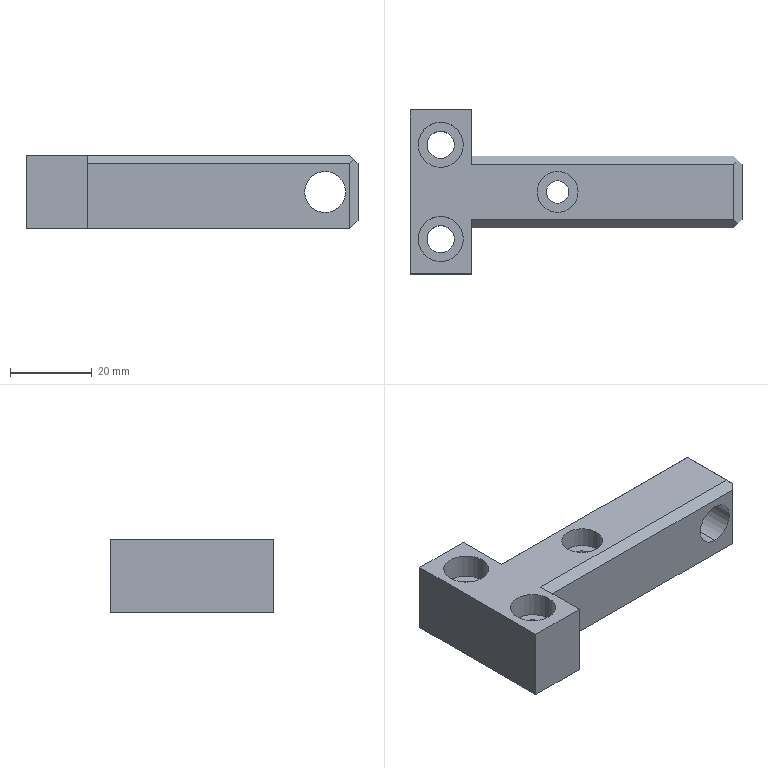Part | NX | features BREP 1 | 1 solid | 33 faces | box 81 x 40 x 18 mm | volume 27164 mm3 | plane 19 | cylinder 14 | commonest cylinder face diameters 6.6 x4 10 x4 11 x4 5.5 x2
STEP:
#1=CARTESIAN_POINT('',(17.428,-446.677,13.));
#2=VERTEX_POINT('',#1);
#3=CARTESIAN_POINT('',(27.428,-446.677,13.));
#4=VERTEX_POINT('',#3);
#5=CARTESIAN_POINT('',(22.428,-446.677,13.));
#6=DIRECTION('',(0.,0.,1.));
#7=DIRECTION('',(1.,0.,0.));
#8=AXIS2_PLACEMENT_3D('',#5,#6,#7);
#9=CIRCLE('',#8,5.);
#10=EDGE_CURVE('',#2,#4,#9,.T.);
#11=ORIENTED_EDGE('',*,*,#10,.F.);
#12=CARTESIAN_POINT('',(17.428,-446.677,18.));
#13=VERTEX_POINT('',#12);
#14=CARTESIAN_POINT('',(17.428,-446.677,18.));
#15=DIRECTION('',(0.,0.,1.));
#16=VECTOR('',#15,1000.);
#17=LINE('',#14,#16);
#18=EDGE_CURVE('',#13,#2,#17,.F.);
#19=ORIENTED_EDGE('',*,*,#18,.F.);
#20=CARTESIAN_POINT('',(27.428,-446.677,18.));
#21=VERTEX_POINT('',#20);
#22=CARTESIAN_POINT('',(22.428,-446.677,18.));
#23=DIRECTION('',(0.,0.,1.));
#24=DIRECTION('',(1.,0.,0.));
#25=AXIS2_PLACEMENT_3D('',#22,#23,#24);
#26=CIRCLE('',#25,5.);
#27=EDGE_CURVE('',#13,#21,#26,.T.);
#28=ORIENTED_EDGE('',*,*,#27,.T.);
#29=CARTESIAN_POINT('',(27.428,-446.677,18.));
#30=DIRECTION('',(0.,0.,1.));
#31=VECTOR('',#30,1000.);
#32=LINE('',#29,#31);
#33=EDGE_CURVE('',#21,#4,#32,.F.);
#34=ORIENTED_EDGE('',*,*,#33,.T.);
#35=EDGE_LOOP('',(#11,#19,#28,#34));
#36=FACE_BOUND('',#35,.T.);
#37=CARTESIAN_POINT('',(22.428,-446.677,18.));
#38=DIRECTION('',(0.,0.,1.));
#39=DIRECTION('',(1.,0.,0.));
#40=AXIS2_PLACEMENT_3D('',#37,#38,#39);
#41=CYLINDRICAL_SURFACE('',#40,5.);
#42=ADVANCED_FACE('',(#36),#41,.F.);
#43=CARTESIAN_POINT('',(19.678,-446.677,0.));
#44=VERTEX_POINT('',#43);
#45=CARTESIAN_POINT('',(25.178,-446.677,0.));
#46=VERTEX_POINT('',#45);
#47=CARTESIAN_POINT('',(22.428,-446.677,0.));
#48=DIRECTION('',(0.,0.,1.));
#49=DIRECTION('',(1.,0.,0.));
#50=AXIS2_PLACEMENT_3D('',#47,#48,#49);
#51=CIRCLE('',#50,2.75);
#52=EDGE_CURVE('',#44,#46,#51,.T.);
#53=ORIENTED_EDGE('',*,*,#52,.F.);
#54=CARTESIAN_POINT('',(19.678,-446.677,13.));
#55=VERTEX_POINT('',#54);
#56=CARTESIAN_POINT('',(19.678,-446.677,18.));
#57=DIRECTION('',(0.,0.,1.));
#58=VECTOR('',#57,1000.);
#59=LINE('',#56,#58);
#60=EDGE_CURVE('',#55,#44,#59,.F.);
#61=ORIENTED_EDGE('',*,*,#60,.F.);
#62=CARTESIAN_POINT('',(25.178,-446.677,13.));
#63=VERTEX_POINT('',#62);
#64=CARTESIAN_POINT('',(22.428,-446.677,13.));
#65=DIRECTION('',(0.,0.,1.));
#66=DIRECTION('',(1.,0.,0.));
#67=AXIS2_PLACEMENT_3D('',#64,#65,#66);
#68=CIRCLE('',#67,2.75);
#69=EDGE_CURVE('',#55,#63,#68,.T.);
#70=ORIENTED_EDGE('',*,*,#69,.T.);
#71=CARTESIAN_POINT('',(25.178,-446.677,18.));
#72=DIRECTION('',(0.,0.,1.));
#73=VECTOR('',#72,1000.);
#74=LINE('',#71,#73);
#75=EDGE_CURVE('',#63,#46,#74,.F.);
#76=ORIENTED_EDGE('',*,*,#75,.T.);
#77=EDGE_LOOP('',(#53,#61,#70,#76));
#78=FACE_BOUND('',#77,.T.);
#79=CARTESIAN_POINT('',(22.428,-446.677,18.));
#80=DIRECTION('',(0.,0.,1.));
#81=DIRECTION('',(1.,0.,0.));
#82=AXIS2_PLACEMENT_3D('',#79,#80,#81);
#83=CYLINDRICAL_SURFACE('',#82,2.75);
#84=ADVANCED_FACE('',(#78),#83,.F.);
#85=CARTESIAN_POINT('',(-11.572,-435.177,12.));
#86=VERTEX_POINT('',#85);
#87=CARTESIAN_POINT('',(-0.5719,-435.177,12.));
#88=VERTEX_POINT('',#87);
#89=CARTESIAN_POINT('',(-6.072,-435.177,12.));
#90=DIRECTION('',(0.,0.,1.));
#91=DIRECTION('',(1.,0.,0.));
#92=AXIS2_PLACEMENT_3D('',#89,#90,#91);
#93=CIRCLE('',#92,5.5);
#94=EDGE_CURVE('',#86,#88,#93,.T.);
#95=ORIENTED_EDGE('',*,*,#94,.F.);
#96=CARTESIAN_POINT('',(-11.572,-435.177,18.));
#97=VERTEX_POINT('',#96);
#98=CARTESIAN_POINT('',(-11.572,-435.177,18.));
#99=DIRECTION('',(0.,0.,1.));
#100=VECTOR('',#99,1000.);
#101=LINE('',#98,#100);
#102=EDGE_CURVE('',#97,#86,#101,.F.);
#103=ORIENTED_EDGE('',*,*,#102,.F.);
#104=CARTESIAN_POINT('',(-0.5719,-435.177,18.));
#105=VERTEX_POINT('',#104);
#106=CARTESIAN_POINT('',(-6.072,-435.177,18.));
#107=DIRECTION('',(0.,0.,1.));
#108=DIRECTION('',(1.,0.,0.));
#109=AXIS2_PLACEMENT_3D('',#106,#107,#108);
#110=CIRCLE('',#109,5.5);
#111=EDGE_CURVE('',#97,#105,#110,.T.);
#112=ORIENTED_EDGE('',*,*,#111,.T.);
#113=CARTESIAN_POINT('',(-0.5719,-435.177,18.));
#114=DIRECTION('',(0.,0.,1.));
#115=VECTOR('',#114,1000.);
#116=LINE('',#113,#115);
#117=EDGE_CURVE('',#105,#88,#116,.F.);
#118=ORIENTED_EDGE('',*,*,#117,.T.);
#119=EDGE_LOOP('',(#95,#103,#112,#118));
#120=FACE_BOUND('',#119,.T.);
#121=CARTESIAN_POINT('',(-6.072,-435.177,18.));
#122=DIRECTION('',(0.,0.,1.));
#123=DIRECTION('',(1.,0.,0.));
#124=AXIS2_PLACEMENT_3D('',#121,#122,#123);
#125=CYLINDRICAL_SURFACE('',#124,5.5);
#126=ADVANCED_FACE('',(#120),#125,.F.);
#127=CARTESIAN_POINT('',(-9.372,-435.177,0.));
#128=VERTEX_POINT('',#127);
#129=CARTESIAN_POINT('',(-2.772,-435.177,0.));
#130=VERTEX_POINT('',#129);
#131=CARTESIAN_POINT('',(-6.072,-435.177,0.));
#132=DIRECTION('',(0.,0.,1.));
#133=DIRECTION('',(1.,0.,0.));
#134=AXIS2_PLACEMENT_3D('',#131,#132,#133);
#135=CIRCLE('',#134,3.3);
#136=EDGE_CURVE('',#128,#130,#135,.T.);
#137=ORIENTED_EDGE('',*,*,#136,.F.);
#138=CARTESIAN_POINT('',(-9.372,-435.177,12.));
#139=VERTEX_POINT('',#138);
#140=CARTESIAN_POINT('',(-9.372,-435.177,18.));
#141=DIRECTION('',(0.,0.,1.));
#142=VECTOR('',#141,1000.);
#143=LINE('',#140,#142);
#144=EDGE_CURVE('',#139,#128,#143,.F.);
#145=ORIENTED_EDGE('',*,*,#144,.F.);
#146=CARTESIAN_POINT('',(-2.772,-435.177,12.));
#147=VERTEX_POINT('',#146);
#148=CARTESIAN_POINT('',(-6.072,-435.177,12.));
#149=DIRECTION('',(0.,0.,1.));
#150=DIRECTION('',(1.,0.,0.));
#151=AXIS2_PLACEMENT_3D('',#148,#149,#150);
#152=CIRCLE('',#151,3.3);
#153=EDGE_CURVE('',#139,#147,#152,.T.);
#154=ORIENTED_EDGE('',*,*,#153,.T.);
#155=CARTESIAN_POINT('',(-2.772,-435.177,18.));
#156=DIRECTION('',(0.,0.,1.));
#157=VECTOR('',#156,1000.);
#158=LINE('',#155,#157);
#159=EDGE_CURVE('',#147,#130,#158,.F.);
#160=ORIENTED_EDGE('',*,*,#159,.T.);
#161=EDGE_LOOP('',(#137,#145,#154,#160));
#162=FACE_BOUND('',#161,.T.);
#163=CARTESIAN_POINT('',(-6.072,-435.177,18.));
#164=DIRECTION('',(0.,0.,1.));
#165=DIRECTION('',(1.,0.,0.));
#166=AXIS2_PLACEMENT_3D('',#163,#164,#165);
#167=CYLINDRICAL_SURFACE('',#166,3.3);
#168=ADVANCED_FACE('',(#162),#167,.F.);
#169=CARTESIAN_POINT('',(-11.572,-458.177,12.));
#170=VERTEX_POINT('',#169);
#171=CARTESIAN_POINT('',(-0.5719,-458.177,12.));
#172=VERTEX_POINT('',#171);
#173=CARTESIAN_POINT('',(-6.072,-458.177,12.));
#174=DIRECTION('',(0.,0.,1.));
#175=DIRECTION('',(1.,0.,0.));
#176=AXIS2_PLACEMENT_3D('',#173,#174,#175);
#177=CIRCLE('',#176,5.5);
#178=EDGE_CURVE('',#170,#172,#177,.T.);
#179=ORIENTED_EDGE('',*,*,#178,.F.);
#180=CARTESIAN_POINT('',(-11.572,-458.177,18.));
#181=VERTEX_POINT('',#180);
#182=CARTESIAN_POINT('',(-11.572,-458.177,18.));
#183=DIRECTION('',(0.,0.,1.));
#184=VECTOR('',#183,1000.);
#185=LINE('',#182,#184);
#186=EDGE_CURVE('',#181,#170,#185,.F.);
#187=ORIENTED_EDGE('',*,*,#186,.F.);
#188=CARTESIAN_POINT('',(-0.5719,-458.177,18.));
#189=VERTEX_POINT('',#188);
#190=CARTESIAN_POINT('',(-6.072,-458.177,18.));
#191=DIRECTION('',(0.,0.,1.));
#192=DIRECTION('',(1.,0.,0.));
#193=AXIS2_PLACEMENT_3D('',#190,#191,#192);
#194=CIRCLE('',#193,5.5);
#195=EDGE_CURVE('',#181,#189,#194,.T.);
#196=ORIENTED_EDGE('',*,*,#195,.T.);
#197=CARTESIAN_POINT('',(-0.5719,-458.177,18.));
#198=DIRECTION('',(0.,0.,1.));
#199=VECTOR('',#198,1000.);
#200=LINE('',#197,#199);
#201=EDGE_CURVE('',#189,#172,#200,.F.);
#202=ORIENTED_EDGE('',*,*,#201,.T.);
#203=EDGE_LOOP('',(#179,#187,#196,#202));
#204=FACE_BOUND('',#203,.T.);
#205=CARTESIAN_POINT('',(-6.072,-458.177,18.));
#206=DIRECTION('',(0.,0.,1.));
#207=DIRECTION('',(1.,0.,0.));
#208=AXIS2_PLACEMENT_3D('',#205,#206,#207);
#209=CYLINDRICAL_SURFACE('',#208,5.5);
#210=ADVANCED_FACE('',(#204),#209,.F.);
#211=CARTESIAN_POINT('',(-9.372,-458.177,0.));
#212=VERTEX_POINT('',#211);
#213=CARTESIAN_POINT('',(-2.772,-458.177,0.));
#214=VERTEX_POINT('',#213);
#215=CARTESIAN_POINT('',(-6.072,-458.177,0.));
#216=DIRECTION('',(0.,0.,1.));
#217=DIRECTION('',(1.,0.,0.));
#218=AXIS2_PLACEMENT_3D('',#215,#216,#217);
#219=CIRCLE('',#218,3.3);
#220=EDGE_CURVE('',#212,#214,#219,.T.);
#221=ORIENTED_EDGE('',*,*,#220,.F.);
#222=CARTESIAN_POINT('',(-9.372,-458.177,12.));
#223=VERTEX_POINT('',#222);
#224=CARTESIAN_POINT('',(-9.372,-458.177,18.));
#225=DIRECTION('',(0.,0.,1.));
#226=VECTOR('',#225,1000.);
#227=LINE('',#224,#226);
#228=EDGE_CURVE('',#223,#212,#227,.F.);
#229=ORIENTED_EDGE('',*,*,#228,.F.);
#230=CARTESIAN_POINT('',(-2.772,-458.177,12.));
#231=VERTEX_POINT('',#230);
#232=CARTESIAN_POINT('',(-6.072,-458.177,12.));
#233=DIRECTION('',(0.,0.,1.));
#234=DIRECTION('',(1.,0.,0.));
#235=AXIS2_PLACEMENT_3D('',#232,#233,#234);
#236=CIRCLE('',#235,3.3);
#237=EDGE_CURVE('',#223,#231,#236,.T.);
#238=ORIENTED_EDGE('',*,*,#237,.T.);
#239=CARTESIAN_POINT('',(-2.772,-458.177,18.));
#240=DIRECTION('',(0.,0.,1.));
#241=VECTOR('',#240,1000.);
#242=LINE('',#239,#241);
#243=EDGE_CURVE('',#231,#214,#242,.F.);
#244=ORIENTED_EDGE('',*,*,#243,.T.);
#245=EDGE_LOOP('',(#221,#229,#238,#244));
#246=FACE_BOUND('',#245,.T.);
#247=CARTESIAN_POINT('',(-6.072,-458.177,18.));
#248=DIRECTION('',(0.,0.,1.));
#249=DIRECTION('',(1.,0.,0.));
#250=AXIS2_PLACEMENT_3D('',#247,#248,#249);
#251=CYLINDRICAL_SURFACE('',#250,3.3);
#252=ADVANCED_FACE('',(#246),#251,.F.);
#253=CARTESIAN_POINT('',(59.428,-437.927,14.));
#254=VERTEX_POINT('',#253);
#255=CARTESIAN_POINT('',(59.428,-437.927,4.));
#256=VERTEX_POINT('',#255);
#257=CARTESIAN_POINT('',(59.428,-437.927,9.));
#258=DIRECTION('',(0.,-1.,0.));
#259=DIRECTION('',(0.,0.,-1.));
#260=AXIS2_PLACEMENT_3D('',#257,#258,#259);
#261=CIRCLE('',#260,5.);
#262=EDGE_CURVE('',#254,#256,#261,.T.);
#263=ORIENTED_EDGE('',*,*,#262,.F.);
#264=CARTESIAN_POINT('',(59.428,-455.427,14.));
#265=VERTEX_POINT('',#264);
#266=CARTESIAN_POINT('',(59.428,-426.677,14.));
#267=DIRECTION('',(0.,-1.,0.));
#268=VECTOR('',#267,1000.);
#269=LINE('',#266,#268);
#270=EDGE_CURVE('',#254,#265,#269,.T.);
#271=ORIENTED_EDGE('',*,*,#270,.T.);
#272=CARTESIAN_POINT('',(59.428,-455.427,4.));
#273=VERTEX_POINT('',#272);
#274=CARTESIAN_POINT('',(59.428,-455.427,9.));
#275=DIRECTION('',(0.,-1.,0.));
#276=DIRECTION('',(0.,0.,-1.));
#277=AXIS2_PLACEMENT_3D('',#274,#275,#276);
#278=CIRCLE('',#277,5.);
#279=EDGE_CURVE('',#265,#273,#278,.T.);
#280=ORIENTED_EDGE('',*,*,#279,.T.);
#281=CARTESIAN_POINT('',(59.428,-426.677,4.));
#282=DIRECTION('',(0.,-1.,0.));
#283=VECTOR('',#282,1000.);
#284=LINE('',#281,#283);
#285=EDGE_CURVE('',#256,#273,#284,.T.);
#286=ORIENTED_EDGE('',*,*,#285,.F.);
#287=EDGE_LOOP('',(#263,#271,#280,#286));
#288=FACE_BOUND('',#287,.T.);
#289=CARTESIAN_POINT('',(59.428,-426.677,9.));
#290=DIRECTION('',(0.,-1.,0.));
#291=DIRECTION('',(0.,0.,-1.));
#292=AXIS2_PLACEMENT_3D('',#289,#290,#291);
#293=CYLINDRICAL_SURFACE('',#292,5.);
#294=ADVANCED_FACE('',(#288),#293,.F.);
#295=CARTESIAN_POINT('',(67.428,-439.927,16.));
#296=VERTEX_POINT('',#295);
#297=CARTESIAN_POINT('',(67.428,-453.427,16.));
#298=VERTEX_POINT('',#297);
#299=CARTESIAN_POINT('',(67.428,-455.427,16.));
#300=DIRECTION('',(0.,-1.,0.));
#301=VECTOR('',#300,1000.);
#302=LINE('',#299,#301);
#303=EDGE_CURVE('',#296,#298,#302,.T.);
#304=ORIENTED_EDGE('',*,*,#303,.T.);
#305=CARTESIAN_POINT('',(67.428,-453.427,2.));
#306=VERTEX_POINT('',#305);
#307=CARTESIAN_POINT('',(67.428,-453.427,18.));
#308=DIRECTION('',(0.,0.,-1.));
#309=VECTOR('',#308,1000.);
#310=LINE('',#307,#309);
#311=EDGE_CURVE('',#298,#306,#310,.T.);
#312=ORIENTED_EDGE('',*,*,#311,.T.);
#313=CARTESIAN_POINT('',(67.428,-439.927,2.));
#314=VERTEX_POINT('',#313);
#315=CARTESIAN_POINT('',(67.428,-437.927,2.));
#316=DIRECTION('',(0.,1.,0.));
#317=VECTOR('',#316,1000.);
#318=LINE('',#315,#317);
#319=EDGE_CURVE('',#306,#314,#318,.T.);
#320=ORIENTED_EDGE('',*,*,#319,.T.);
#321=CARTESIAN_POINT('',(67.428,-439.927,18.));
#322=DIRECTION('',(0.,0.,1.));
#323=VECTOR('',#322,1000.);
#324=LINE('',#321,#323);
#325=EDGE_CURVE('',#314,#296,#324,.T.);
#326=ORIENTED_EDGE('',*,*,#325,.T.);
#327=EDGE_LOOP('',(#304,#312,#320,#326));
#328=FACE_BOUND('',#327,.T.);
#329=CARTESIAN_POINT('',(67.428,-437.927,18.));
#330=DIRECTION('',(-1.,0.,0.));
#331=DIRECTION('',(0.,0.,1.));
#332=AXIS2_PLACEMENT_3D('',#329,#330,#331);
#333=PLANE('',#332);
#334=ADVANCED_FACE('',(#328),#333,.F.);
#335=CARTESIAN_POINT('',(1.428,-437.927,16.));
#336=VERTEX_POINT('',#335);
#337=CARTESIAN_POINT('',(1.428,-437.927,0.));
#338=VERTEX_POINT('',#337);
#339=CARTESIAN_POINT('',(1.428,-437.927,18.));
#340=DIRECTION('',(0.,0.,-1.));
#341=VECTOR('',#340,1000.);
#342=LINE('',#339,#341);
#343=EDGE_CURVE('',#336,#338,#342,.T.);
#344=ORIENTED_EDGE('',*,*,#343,.F.);
#345=CARTESIAN_POINT('',(65.428,-437.927,16.));
#346=VERTEX_POINT('',#345);
#347=CARTESIAN_POINT('',(65.428,-437.927,16.));
#348=DIRECTION('',(1.,0.,0.));
#349=VECTOR('',#348,1000.);
#350=LINE('',#347,#349);
#351=EDGE_CURVE('',#336,#346,#350,.T.);
#352=ORIENTED_EDGE('',*,*,#351,.T.);
#353=CARTESIAN_POINT('',(65.428,-437.927,0.));
#354=VERTEX_POINT('',#353);
#355=CARTESIAN_POINT('',(65.428,-437.927,18.));
#356=DIRECTION('',(0.,0.,-1.));
#357=VECTOR('',#356,1000.);
#358=LINE('',#355,#357);
#359=EDGE_CURVE('',#346,#354,#358,.T.);
#360=ORIENTED_EDGE('',*,*,#359,.T.);
#361=CARTESIAN_POINT('',(1.428,-437.927,0.));
#362=DIRECTION('',(-1.,0.,0.));
#363=VECTOR('',#362,1000.);
#364=LINE('',#361,#363);
#365=EDGE_CURVE('',#354,#338,#364,.T.);
#366=ORIENTED_EDGE('',*,*,#365,.T.);
#367=EDGE_LOOP('',(#344,#352,#360,#366));
#368=FACE_BOUND('',#367,.T.);
#369=CARTESIAN_POINT('',(59.428,-437.927,9.));
#370=DIRECTION('',(0.,-1.,0.));
#371=DIRECTION('',(0.,0.,-1.));
#372=AXIS2_PLACEMENT_3D('',#369,#370,#371);
#373=CIRCLE('',#372,5.);
#374=EDGE_CURVE('',#256,#254,#373,.T.);
#375=ORIENTED_EDGE('',*,*,#374,.T.);
#376=ORIENTED_EDGE('',*,*,#262,.T.);
#377=EDGE_LOOP('',(#375,#376));
#378=FACE_BOUND('',#377,.T.);
#379=CARTESIAN_POINT('',(1.428,-437.927,18.));
#380=DIRECTION('',(0.,-1.,0.));
#381=DIRECTION('',(0.,0.,-1.));
#382=AXIS2_PLACEMENT_3D('',#379,#380,#381);
#383=PLANE('',#382);
#384=ADVANCED_FACE('',(#368,#378),#383,.F.);
#385=CARTESIAN_POINT('',(1.428,-426.677,0.));
#386=VERTEX_POINT('',#385);
#387=CARTESIAN_POINT('',(1.428,-437.927,0.));
#388=DIRECTION('',(0.,1.,0.));
#389=VECTOR('',#388,1000.);
#390=LINE('',#387,#389);
#391=EDGE_CURVE('',#338,#386,#390,.T.);
#392=ORIENTED_EDGE('',*,*,#391,.T.);
#393=CARTESIAN_POINT('',(1.428,-426.677,18.));
#394=VERTEX_POINT('',#393);
#395=CARTESIAN_POINT('',(1.428,-426.677,18.));
#396=DIRECTION('',(0.,0.,-1.));
#397=VECTOR('',#396,1000.);
#398=LINE('',#395,#397);
#399=EDGE_CURVE('',#394,#386,#398,.T.);
#400=ORIENTED_EDGE('',*,*,#399,.F.);
#401=CARTESIAN_POINT('',(1.428,-439.927,18.));
#402=VERTEX_POINT('',#401);
#403=CARTESIAN_POINT('',(1.428,-437.927,18.));
#404=DIRECTION('',(0.,1.,0.));
#405=VECTOR('',#404,1000.);
#406=LINE('',#403,#405);
#407=EDGE_CURVE('',#402,#394,#406,.T.);
#408=ORIENTED_EDGE('',*,*,#407,.F.);
#409=CARTESIAN_POINT('',(1.428,-438.927,17.));
#410=DIRECTION('',(0.,0.7071,-0.7071));
#411=VECTOR('',#410,1000.);
#412=LINE('',#409,#411);
#413=EDGE_CURVE('',#402,#336,#412,.T.);
#414=ORIENTED_EDGE('',*,*,#413,.T.);
#415=ORIENTED_EDGE('',*,*,#343,.T.);
#416=EDGE_LOOP('',(#392,#400,#408,#414,#415));
#417=FACE_BOUND('',#416,.T.);
#418=CARTESIAN_POINT('',(1.428,-437.927,18.));
#419=DIRECTION('',(-1.,0.,0.));
#420=DIRECTION('',(0.,0.,1.));
#421=AXIS2_PLACEMENT_3D('',#418,#419,#420);
#422=PLANE('',#421);
#423=ADVANCED_FACE('',(#417),#422,.F.);
#424=CARTESIAN_POINT('',(-13.572,-426.677,0.));
#425=VERTEX_POINT('',#424);
#426=CARTESIAN_POINT('',(-13.572,-426.677,0.));
#427=DIRECTION('',(-1.,0.,0.));
#428=VECTOR('',#427,1000.);
#429=LINE('',#426,#428);
#430=EDGE_CURVE('',#386,#425,#429,.T.);
#431=ORIENTED_EDGE('',*,*,#430,.T.);
#432=CARTESIAN_POINT('',(-13.572,-426.677,18.));
#433=VERTEX_POINT('',#432);
#434=CARTESIAN_POINT('',(-13.572,-426.677,18.));
#435=DIRECTION('',(0.,0.,-1.));
#436=VECTOR('',#435,1000.);
#437=LINE('',#434,#436);
#438=EDGE_CURVE('',#433,#425,#437,.T.);
#439=ORIENTED_EDGE('',*,*,#438,.F.);
#440=CARTESIAN_POINT('',(-13.572,-426.677,18.));
#441=DIRECTION('',(-1.,0.,0.));
#442=VECTOR('',#441,1000.);
#443=LINE('',#440,#442);
#444=EDGE_CURVE('',#394,#433,#443,.T.);
#445=ORIENTED_EDGE('',*,*,#444,.F.);
#446=ORIENTED_EDGE('',*,*,#399,.T.);
#447=EDGE_LOOP('',(#431,#439,#445,#446));
#448=FACE_BOUND('',#447,.T.);
#449=CARTESIAN_POINT('',(-13.572,-426.677,18.));
#450=DIRECTION('',(0.,-1.,0.));
#451=DIRECTION('',(0.,0.,-1.));
#452=AXIS2_PLACEMENT_3D('',#449,#450,#451);
#453=PLANE('',#452);
#454=ADVANCED_FACE('',(#448),#453,.F.);
#455=CARTESIAN_POINT('',(-13.572,-466.677,0.));
#456=VERTEX_POINT('',#455);
#457=CARTESIAN_POINT('',(-13.572,-449.911,0.));
#458=DIRECTION('',(0.,-1.,0.));
#459=VECTOR('',#458,1000.);
#460=LINE('',#457,#459);
#461=EDGE_CURVE('',#425,#456,#460,.T.);
#462=ORIENTED_EDGE('',*,*,#461,.T.);
#463=CARTESIAN_POINT('',(-13.572,-466.677,18.));
#464=VERTEX_POINT('',#463);
#465=CARTESIAN_POINT('',(-13.572,-466.677,18.));
#466=DIRECTION('',(0.,0.,-1.));
#467=VECTOR('',#466,1000.);
#468=LINE('',#465,#467);
#469=EDGE_CURVE('',#464,#456,#468,.T.);
#470=ORIENTED_EDGE('',*,*,#469,.F.);
#471=CARTESIAN_POINT('',(-13.572,-449.911,18.));
#472=DIRECTION('',(0.,-1.,0.));
#473=VECTOR('',#472,1000.);
#474=LINE('',#471,#473);
#475=EDGE_CURVE('',#433,#464,#474,.T.);
#476=ORIENTED_EDGE('',*,*,#475,.F.);
#477=ORIENTED_EDGE('',*,*,#438,.T.);
#478=EDGE_LOOP('',(#462,#470,#476,#477));
#479=FACE_BOUND('',#478,.T.);
#480=CARTESIAN_POINT('',(-13.572,-449.911,18.));
#481=DIRECTION('',(1.,0.,0.));
#482=DIRECTION('',(0.,1.,0.));
#483=AXIS2_PLACEMENT_3D('',#480,#481,#482);
#484=PLANE('',#483);
#485=ADVANCED_FACE('',(#479),#484,.F.);
#486=CARTESIAN_POINT('',(1.428,-466.677,0.));
#487=VERTEX_POINT('',#486);
#488=CARTESIAN_POINT('',(-13.572,-466.677,0.));
#489=DIRECTION('',(1.,0.,0.));
#490=VECTOR('',#489,1000.);
#491=LINE('',#488,#490);
#492=EDGE_CURVE('',#456,#487,#491,.T.);
#493=ORIENTED_EDGE('',*,*,#492,.T.);
#494=CARTESIAN_POINT('',(1.428,-466.677,18.));
#495=VERTEX_POINT('',#494);
#496=CARTESIAN_POINT('',(1.428,-466.677,18.));
#497=DIRECTION('',(0.,0.,-1.));
#498=VECTOR('',#497,1000.);
#499=LINE('',#496,#498);
#500=EDGE_CURVE('',#495,#487,#499,.T.);
#501=ORIENTED_EDGE('',*,*,#500,.F.);
#502=CARTESIAN_POINT('',(-13.572,-466.677,18.));
#503=DIRECTION('',(1.,0.,0.));
#504=VECTOR('',#503,1000.);
#505=LINE('',#502,#504);
#506=EDGE_CURVE('',#464,#495,#505,.T.);
#507=ORIENTED_EDGE('',*,*,#506,.F.);
#508=ORIENTED_EDGE('',*,*,#469,.T.);
#509=EDGE_LOOP('',(#493,#501,#507,#508));
#510=FACE_BOUND('',#509,.T.);
#511=CARTESIAN_POINT('',(-13.572,-466.677,18.));
#512=DIRECTION('',(0.,1.,0.));
#513=DIRECTION('',(1.,0.,0.));
#514=AXIS2_PLACEMENT_3D('',#511,#512,#513);
#515=PLANE('',#514);
#516=ADVANCED_FACE('',(#510),#515,.F.);
#517=CARTESIAN_POINT('',(1.428,-455.427,0.));
#518=VERTEX_POINT('',#517);
#519=CARTESIAN_POINT('',(1.428,-455.427,0.));
#520=DIRECTION('',(0.,1.,0.));
#521=VECTOR('',#520,1000.);
#522=LINE('',#519,#521);
#523=EDGE_CURVE('',#487,#518,#522,.T.);
#524=ORIENTED_EDGE('',*,*,#523,.T.);
#525=CARTESIAN_POINT('',(1.428,-455.427,16.));
#526=VERTEX_POINT('',#525);
#527=CARTESIAN_POINT('',(1.428,-455.427,18.));
#528=DIRECTION('',(0.,0.,-1.));
#529=VECTOR('',#528,1000.);
#530=LINE('',#527,#529);
#531=EDGE_CURVE('',#526,#518,#530,.T.);
#532=ORIENTED_EDGE('',*,*,#531,.F.);
#533=CARTESIAN_POINT('',(1.428,-453.427,18.));
#534=VERTEX_POINT('',#533);
#535=CARTESIAN_POINT('',(1.428,-454.427,17.));
#536=DIRECTION('',(0.,0.7071,0.7071));
#537=VECTOR('',#536,1000.);
#538=LINE('',#535,#537);
#539=EDGE_CURVE('',#526,#534,#538,.T.);
#540=ORIENTED_EDGE('',*,*,#539,.T.);
#541=CARTESIAN_POINT('',(1.428,-455.427,18.));
#542=DIRECTION('',(0.,1.,0.));
#543=VECTOR('',#542,1000.);
#544=LINE('',#541,#543);
#545=EDGE_CURVE('',#495,#534,#544,.T.);
#546=ORIENTED_EDGE('',*,*,#545,.F.);
#547=ORIENTED_EDGE('',*,*,#500,.T.);
#548=EDGE_LOOP('',(#524,#532,#540,#546,#547));
#549=FACE_BOUND('',#548,.T.);
#550=CARTESIAN_POINT('',(1.428,-455.427,18.));
#551=DIRECTION('',(-1.,0.,0.));
#552=DIRECTION('',(0.,0.,1.));
#553=AXIS2_PLACEMENT_3D('',#550,#551,#552);
#554=PLANE('',#553);
#555=ADVANCED_FACE('',(#549),#554,.F.);
#556=CARTESIAN_POINT('',(65.428,-455.427,0.));
#557=VERTEX_POINT('',#556);
#558=CARTESIAN_POINT('',(65.428,-455.427,16.));
#559=VERTEX_POINT('',#558);
#560=CARTESIAN_POINT('',(65.428,-455.427,18.));
#561=DIRECTION('',(0.,0.,1.));
#562=VECTOR('',#561,1000.);
#563=LINE('',#560,#562);
#564=EDGE_CURVE('',#557,#559,#563,.T.);
#565=ORIENTED_EDGE('',*,*,#564,.T.);
#566=CARTESIAN_POINT('',(1.428,-455.427,16.));
#567=DIRECTION('',(-1.,0.,0.));
#568=VECTOR('',#567,1000.);
#569=LINE('',#566,#568);
#570=EDGE_CURVE('',#559,#526,#569,.T.);
#571=ORIENTED_EDGE('',*,*,#570,.T.);
#572=ORIENTED_EDGE('',*,*,#531,.T.);
#573=CARTESIAN_POINT('',(1.428,-455.427,0.));
#574=DIRECTION('',(1.,0.,0.));
#575=VECTOR('',#574,1000.);
#576=LINE('',#573,#575);
#577=EDGE_CURVE('',#518,#557,#576,.T.);
#578=ORIENTED_EDGE('',*,*,#577,.T.);
#579=EDGE_LOOP('',(#565,#571,#572,#578));
#580=FACE_BOUND('',#579,.T.);
#581=CARTESIAN_POINT('',(59.428,-455.427,9.));
#582=DIRECTION('',(0.,-1.,0.));
#583=DIRECTION('',(0.,0.,-1.));
#584=AXIS2_PLACEMENT_3D('',#581,#582,#583);
#585=CIRCLE('',#584,5.);
#586=EDGE_CURVE('',#273,#265,#585,.T.);
#587=ORIENTED_EDGE('',*,*,#586,.F.);
#588=ORIENTED_EDGE('',*,*,#279,.F.);
#589=EDGE_LOOP('',(#587,#588));
#590=FACE_BOUND('',#589,.T.);
#591=CARTESIAN_POINT('',(1.428,-455.427,18.));
#592=DIRECTION('',(0.,1.,0.));
#593=DIRECTION('',(1.,0.,0.));
#594=AXIS2_PLACEMENT_3D('',#591,#592,#593);
#595=PLANE('',#594);
#596=ADVANCED_FACE('',(#580,#590),#595,.F.);
#597=ORIENTED_EDGE('',*,*,#545,.T.);
#598=CARTESIAN_POINT('',(65.428,-453.427,18.));
#599=VERTEX_POINT('',#598);
#600=CARTESIAN_POINT('',(65.428,-453.427,18.));
#601=DIRECTION('',(1.,0.,0.));
#602=VECTOR('',#601,1000.);
#603=LINE('',#600,#602);
#604=EDGE_CURVE('',#534,#599,#603,.T.);
#605=ORIENTED_EDGE('',*,*,#604,.T.);
#606=CARTESIAN_POINT('',(65.428,-439.927,18.));
#607=VERTEX_POINT('',#606);
#608=CARTESIAN_POINT('',(65.428,-437.927,18.));
#609=DIRECTION('',(0.,1.,0.));
#610=VECTOR('',#609,1000.);
#611=LINE('',#608,#610);
#612=EDGE_CURVE('',#599,#607,#611,.T.);
#613=ORIENTED_EDGE('',*,*,#612,.T.);
#614=CARTESIAN_POINT('',(1.428,-439.927,18.));
#615=DIRECTION('',(-1.,0.,0.));
#616=VECTOR('',#615,1000.);
#617=LINE('',#614,#616);
#618=EDGE_CURVE('',#607,#402,#617,.T.);
#619=ORIENTED_EDGE('',*,*,#618,.T.);
#620=ORIENTED_EDGE('',*,*,#407,.T.);
#621=ORIENTED_EDGE('',*,*,#444,.T.);
#622=ORIENTED_EDGE('',*,*,#475,.T.);
#623=ORIENTED_EDGE('',*,*,#506,.T.);
#624=EDGE_LOOP('',(#597,#605,#613,#619,#620,#621,#622,#623));
#625=FACE_BOUND('',#624,.T.);
#626=CARTESIAN_POINT('',(22.428,-446.677,18.));
#627=DIRECTION('',(0.,0.,1.));
#628=DIRECTION('',(1.,0.,0.));
#629=AXIS2_PLACEMENT_3D('',#626,#627,#628);
#630=CIRCLE('',#629,5.);
#631=EDGE_CURVE('',#21,#13,#630,.T.);
#632=ORIENTED_EDGE('',*,*,#631,.F.);
#633=ORIENTED_EDGE('',*,*,#27,.F.);
#634=EDGE_LOOP('',(#632,#633));
#635=FACE_BOUND('',#634,.T.);
#636=CARTESIAN_POINT('',(-6.072,-435.177,18.));
#637=DIRECTION('',(0.,0.,1.));
#638=DIRECTION('',(1.,0.,0.));
#639=AXIS2_PLACEMENT_3D('',#636,#637,#638);
#640=CIRCLE('',#639,5.5);
#641=EDGE_CURVE('',#105,#97,#640,.T.);
#642=ORIENTED_EDGE('',*,*,#641,.F.);
#643=ORIENTED_EDGE('',*,*,#111,.F.);
#644=EDGE_LOOP('',(#642,#643));
#645=FACE_BOUND('',#644,.T.);
#646=CARTESIAN_POINT('',(-6.072,-458.177,18.));
#647=DIRECTION('',(0.,0.,1.));
#648=DIRECTION('',(1.,0.,0.));
#649=AXIS2_PLACEMENT_3D('',#646,#647,#648);
#650=CIRCLE('',#649,5.5);
#651=EDGE_CURVE('',#189,#181,#650,.T.);
#652=ORIENTED_EDGE('',*,*,#651,.F.);
#653=ORIENTED_EDGE('',*,*,#195,.F.);
#654=EDGE_LOOP('',(#652,#653));
#655=FACE_BOUND('',#654,.T.);
#656=CARTESIAN_POINT('',(67.428,-455.427,18.));
#657=DIRECTION('',(0.,0.,1.));
#658=DIRECTION('',(1.,0.,0.));
#659=AXIS2_PLACEMENT_3D('',#656,#657,#658);
#660=PLANE('',#659);
#661=ADVANCED_FACE('',(#625,#635,#645,#655),#660,.T.);
#662=ORIENTED_EDGE('',*,*,#365,.F.);
#663=CARTESIAN_POINT('',(65.428,-455.427,0.));
#664=DIRECTION('',(0.,-1.,0.));
#665=VECTOR('',#664,1000.);
#666=LINE('',#663,#665);
#667=EDGE_CURVE('',#354,#557,#666,.T.);
#668=ORIENTED_EDGE('',*,*,#667,.T.);
#669=ORIENTED_EDGE('',*,*,#577,.F.);
#670=ORIENTED_EDGE('',*,*,#523,.F.);
#671=ORIENTED_EDGE('',*,*,#492,.F.);
#672=ORIENTED_EDGE('',*,*,#461,.F.);
#673=ORIENTED_EDGE('',*,*,#430,.F.);
#674=ORIENTED_EDGE('',*,*,#391,.F.);
#675=EDGE_LOOP('',(#662,#668,#669,#670,#671,#672,#673,#674));
#676=FACE_BOUND('',#675,.T.);
#677=CARTESIAN_POINT('',(22.428,-446.677,0.));
#678=DIRECTION('',(0.,0.,1.));
#679=DIRECTION('',(1.,0.,0.));
#680=AXIS2_PLACEMENT_3D('',#677,#678,#679);
#681=CIRCLE('',#680,2.75);
#682=EDGE_CURVE('',#46,#44,#681,.T.);
#683=ORIENTED_EDGE('',*,*,#682,.T.);
#684=ORIENTED_EDGE('',*,*,#52,.T.);
#685=EDGE_LOOP('',(#683,#684));
#686=FACE_BOUND('',#685,.T.);
#687=CARTESIAN_POINT('',(-6.072,-435.177,0.));
#688=DIRECTION('',(0.,0.,1.));
#689=DIRECTION('',(1.,0.,0.));
#690=AXIS2_PLACEMENT_3D('',#687,#688,#689);
#691=CIRCLE('',#690,3.3);
#692=EDGE_CURVE('',#130,#128,#691,.T.);
#693=ORIENTED_EDGE('',*,*,#692,.T.);
#694=ORIENTED_EDGE('',*,*,#136,.T.);
#695=EDGE_LOOP('',(#693,#694));
#696=FACE_BOUND('',#695,.T.);
#697=CARTESIAN_POINT('',(-6.072,-458.177,0.));
#698=DIRECTION('',(0.,0.,1.));
#699=DIRECTION('',(1.,0.,0.));
#700=AXIS2_PLACEMENT_3D('',#697,#698,#699);
#701=CIRCLE('',#700,3.3);
#702=EDGE_CURVE('',#214,#212,#701,.T.);
#703=ORIENTED_EDGE('',*,*,#702,.T.);
#704=ORIENTED_EDGE('',*,*,#220,.T.);
#705=EDGE_LOOP('',(#703,#704));
#706=FACE_BOUND('',#705,.T.);
#707=CARTESIAN_POINT('',(67.428,-455.427,0.));
#708=DIRECTION('',(0.,0.,1.));
#709=DIRECTION('',(1.,0.,0.));
#710=AXIS2_PLACEMENT_3D('',#707,#708,#709);
#711=PLANE('',#710);
#712=ADVANCED_FACE('',(#676,#686,#696,#706),#711,.F.);
#713=ORIENTED_EDGE('',*,*,#270,.F.);
#714=ORIENTED_EDGE('',*,*,#374,.F.);
#715=ORIENTED_EDGE('',*,*,#285,.T.);
#716=ORIENTED_EDGE('',*,*,#586,.T.);
#717=EDGE_LOOP('',(#713,#714,#715,#716));
#718=FACE_BOUND('',#717,.T.);
#719=CARTESIAN_POINT('',(59.428,-426.677,9.));
#720=DIRECTION('',(0.,-1.,0.));
#721=DIRECTION('',(0.,0.,-1.));
#722=AXIS2_PLACEMENT_3D('',#719,#720,#721);
#723=CYLINDRICAL_SURFACE('',#722,5.);
#724=ADVANCED_FACE('',(#718),#723,.F.);
#725=ORIENTED_EDGE('',*,*,#228,.T.);
#726=ORIENTED_EDGE('',*,*,#702,.F.);
#727=ORIENTED_EDGE('',*,*,#243,.F.);
#728=CARTESIAN_POINT('',(-6.072,-458.177,12.));
#729=DIRECTION('',(0.,0.,1.));
#730=DIRECTION('',(1.,0.,0.));
#731=AXIS2_PLACEMENT_3D('',#728,#729,#730);
#732=CIRCLE('',#731,3.3);
#733=EDGE_CURVE('',#231,#223,#732,.T.);
#734=ORIENTED_EDGE('',*,*,#733,.T.);
#735=EDGE_LOOP('',(#725,#726,#727,#734));
#736=FACE_BOUND('',#735,.T.);
#737=CARTESIAN_POINT('',(-6.072,-458.177,18.));
#738=DIRECTION('',(0.,0.,1.));
#739=DIRECTION('',(1.,0.,0.));
#740=AXIS2_PLACEMENT_3D('',#737,#738,#739);
#741=CYLINDRICAL_SURFACE('',#740,3.3);
#742=ADVANCED_FACE('',(#736),#741,.F.);
#743=CARTESIAN_POINT('',(-6.072,-458.177,12.));
#744=DIRECTION('',(0.,0.,1.));
#745=DIRECTION('',(1.,0.,0.));
#746=AXIS2_PLACEMENT_3D('',#743,#744,#745);
#747=CIRCLE('',#746,5.5);
#748=EDGE_CURVE('',#172,#170,#747,.T.);
#749=ORIENTED_EDGE('',*,*,#748,.T.);
#750=ORIENTED_EDGE('',*,*,#178,.T.);
#751=EDGE_LOOP('',(#749,#750));
#752=FACE_BOUND('',#751,.T.);
#753=ORIENTED_EDGE('',*,*,#733,.F.);
#754=ORIENTED_EDGE('',*,*,#237,.F.);
#755=EDGE_LOOP('',(#753,#754));
#756=FACE_BOUND('',#755,.T.);
#757=CARTESIAN_POINT('',(-2.772,-458.177,12.));
#758=DIRECTION('',(0.,0.,-1.));
#759=DIRECTION('',(0.,-1.,0.));
#760=AXIS2_PLACEMENT_3D('',#757,#758,#759);
#761=PLANE('',#760);
#762=ADVANCED_FACE('',(#752,#756),#761,.F.);
#763=ORIENTED_EDGE('',*,*,#186,.T.);
#764=ORIENTED_EDGE('',*,*,#748,.F.);
#765=ORIENTED_EDGE('',*,*,#201,.F.);
#766=ORIENTED_EDGE('',*,*,#651,.T.);
#767=EDGE_LOOP('',(#763,#764,#765,#766));
#768=FACE_BOUND('',#767,.T.);
#769=CARTESIAN_POINT('',(-6.072,-458.177,18.));
#770=DIRECTION('',(0.,0.,1.));
#771=DIRECTION('',(1.,0.,0.));
#772=AXIS2_PLACEMENT_3D('',#769,#770,#771);
#773=CYLINDRICAL_SURFACE('',#772,5.5);
#774=ADVANCED_FACE('',(#768),#773,.F.);
#775=ORIENTED_EDGE('',*,*,#144,.T.);
#776=ORIENTED_EDGE('',*,*,#692,.F.);
#777=ORIENTED_EDGE('',*,*,#159,.F.);
#778=CARTESIAN_POINT('',(-6.072,-435.177,12.));
#779=DIRECTION('',(0.,0.,1.));
#780=DIRECTION('',(1.,0.,0.));
#781=AXIS2_PLACEMENT_3D('',#778,#779,#780);
#782=CIRCLE('',#781,3.3);
#783=EDGE_CURVE('',#147,#139,#782,.T.);
#784=ORIENTED_EDGE('',*,*,#783,.T.);
#785=EDGE_LOOP('',(#775,#776,#777,#784));
#786=FACE_BOUND('',#785,.T.);
#787=CARTESIAN_POINT('',(-6.072,-435.177,18.));
#788=DIRECTION('',(0.,0.,1.));
#789=DIRECTION('',(1.,0.,0.));
#790=AXIS2_PLACEMENT_3D('',#787,#788,#789);
#791=CYLINDRICAL_SURFACE('',#790,3.3);
#792=ADVANCED_FACE('',(#786),#791,.F.);
#793=CARTESIAN_POINT('',(-6.072,-435.177,12.));
#794=DIRECTION('',(0.,0.,1.));
#795=DIRECTION('',(1.,0.,0.));
#796=AXIS2_PLACEMENT_3D('',#793,#794,#795);
#797=CIRCLE('',#796,5.5);
#798=EDGE_CURVE('',#88,#86,#797,.T.);
#799=ORIENTED_EDGE('',*,*,#798,.T.);
#800=ORIENTED_EDGE('',*,*,#94,.T.);
#801=EDGE_LOOP('',(#799,#800));
#802=FACE_BOUND('',#801,.T.);
#803=ORIENTED_EDGE('',*,*,#783,.F.);
#804=ORIENTED_EDGE('',*,*,#153,.F.);
#805=EDGE_LOOP('',(#803,#804));
#806=FACE_BOUND('',#805,.T.);
#807=CARTESIAN_POINT('',(-2.772,-435.177,12.));
#808=DIRECTION('',(0.,0.,-1.));
#809=DIRECTION('',(0.,-1.,0.));
#810=AXIS2_PLACEMENT_3D('',#807,#808,#809);
#811=PLANE('',#810);
#812=ADVANCED_FACE('',(#802,#806),#811,.F.);
#813=ORIENTED_EDGE('',*,*,#102,.T.);
#814=ORIENTED_EDGE('',*,*,#798,.F.);
#815=ORIENTED_EDGE('',*,*,#117,.F.);
#816=ORIENTED_EDGE('',*,*,#641,.T.);
#817=EDGE_LOOP('',(#813,#814,#815,#816));
#818=FACE_BOUND('',#817,.T.);
#819=CARTESIAN_POINT('',(-6.072,-435.177,18.));
#820=DIRECTION('',(0.,0.,1.));
#821=DIRECTION('',(1.,0.,0.));
#822=AXIS2_PLACEMENT_3D('',#819,#820,#821);
#823=CYLINDRICAL_SURFACE('',#822,5.5);
#824=ADVANCED_FACE('',(#818),#823,.F.);
#825=ORIENTED_EDGE('',*,*,#359,.F.);
#826=CARTESIAN_POINT('',(66.428,-438.927,17.));
#827=VERTEX_POINT('',#826);
#828=CARTESIAN_POINT('',(66.095,-438.593,16.667));
#829=DIRECTION('',(0.5774,-0.5774,0.5774));
#830=VECTOR('',#829,1000.);
#831=LINE('',#828,#830);
#832=EDGE_CURVE('',#346,#827,#831,.T.);
#833=ORIENTED_EDGE('',*,*,#832,.T.);
#834=CARTESIAN_POINT('',(65.428,-437.927,18.));
#835=DIRECTION('',(-0.5774,0.5774,0.5774));
#836=VECTOR('',#835,1000.);
#837=LINE('',#834,#836);
#838=EDGE_CURVE('',#296,#827,#837,.T.);
#839=ORIENTED_EDGE('',*,*,#838,.F.);
#840=ORIENTED_EDGE('',*,*,#325,.F.);
#841=CARTESIAN_POINT('',(66.761,-439.26,1.333));
#842=DIRECTION('',(0.5774,-0.5774,0.5774));
#843=VECTOR('',#842,1000.);
#844=LINE('',#841,#843);
#845=EDGE_CURVE('',#354,#314,#844,.T.);
#846=ORIENTED_EDGE('',*,*,#845,.F.);
#847=EDGE_LOOP('',(#825,#833,#839,#840,#846));
#848=FACE_BOUND('',#847,.T.);
#849=CARTESIAN_POINT('',(65.428,-437.927,18.));
#850=DIRECTION('',(-0.7071,-0.7071,0.));
#851=DIRECTION('',(-0.7071,0.7071,0.));
#852=AXIS2_PLACEMENT_3D('',#849,#850,#851);
#853=PLANE('',#852);
#854=ADVANCED_FACE('',(#848),#853,.F.);
#855=ORIENTED_EDGE('',*,*,#612,.F.);
#856=CARTESIAN_POINT('',(66.428,-454.427,17.));
#857=VERTEX_POINT('',#856);
#858=CARTESIAN_POINT('',(66.095,-454.093,17.333));
#859=DIRECTION('',(0.5774,-0.5774,-0.5774));
#860=VECTOR('',#859,1000.);
#861=LINE('',#858,#860);
#862=EDGE_CURVE('',#599,#857,#861,.T.);
#863=ORIENTED_EDGE('',*,*,#862,.T.);
#864=CARTESIAN_POINT('',(65.428,-455.427,18.));
#865=DIRECTION('',(-0.5774,-0.5774,0.5774));
#866=VECTOR('',#865,1000.);
#867=LINE('',#864,#866);
#868=EDGE_CURVE('',#298,#857,#867,.T.);
#869=ORIENTED_EDGE('',*,*,#868,.F.);
#870=ORIENTED_EDGE('',*,*,#303,.F.);
#871=ORIENTED_EDGE('',*,*,#838,.T.);
#872=CARTESIAN_POINT('',(60.261,-445.093,23.167));
#873=DIRECTION('',(-0.5774,-0.5774,0.5774));
#874=VECTOR('',#873,1000.);
#875=LINE('',#872,#874);
#876=EDGE_CURVE('',#827,#607,#875,.T.);
#877=ORIENTED_EDGE('',*,*,#876,.T.);
#878=EDGE_LOOP('',(#855,#863,#869,#870,#871,#877));
#879=FACE_BOUND('',#878,.T.);
#880=CARTESIAN_POINT('',(65.428,-455.427,18.));
#881=DIRECTION('',(0.7071,0.,0.7071));
#882=DIRECTION('',(0.,-1.,0.));
#883=AXIS2_PLACEMENT_3D('',#880,#881,#882);
#884=PLANE('',#883);
#885=ADVANCED_FACE('',(#879),#884,.T.);
#886=ORIENTED_EDGE('',*,*,#845,.T.);
#887=ORIENTED_EDGE('',*,*,#319,.F.);
#888=CARTESIAN_POINT('',(72.595,-448.26,7.167));
#889=DIRECTION('',(0.5774,0.5774,0.5774));
#890=VECTOR('',#889,1000.);
#891=LINE('',#888,#890);
#892=EDGE_CURVE('',#557,#306,#891,.T.);
#893=ORIENTED_EDGE('',*,*,#892,.F.);
#894=ORIENTED_EDGE('',*,*,#667,.F.);
#895=EDGE_LOOP('',(#886,#887,#893,#894));
#896=FACE_BOUND('',#895,.T.);
#897=CARTESIAN_POINT('',(67.428,-437.927,2.));
#898=DIRECTION('',(-0.7071,0.,0.7071));
#899=DIRECTION('',(0.,1.,0.));
#900=AXIS2_PLACEMENT_3D('',#897,#898,#899);
#901=PLANE('',#900);
#902=ADVANCED_FACE('',(#896),#901,.F.);
#903=ORIENTED_EDGE('',*,*,#868,.T.);
#904=CARTESIAN_POINT('',(67.428,-453.427,18.));
#905=DIRECTION('',(-0.5774,-0.5774,-0.5774));
#906=VECTOR('',#905,1000.);
#907=LINE('',#904,#906);
#908=EDGE_CURVE('',#857,#559,#907,.T.);
#909=ORIENTED_EDGE('',*,*,#908,.T.);
#910=ORIENTED_EDGE('',*,*,#564,.F.);
#911=ORIENTED_EDGE('',*,*,#892,.T.);
#912=ORIENTED_EDGE('',*,*,#311,.F.);
#913=EDGE_LOOP('',(#903,#909,#910,#911,#912));
#914=FACE_BOUND('',#913,.T.);
#915=CARTESIAN_POINT('',(67.428,-453.427,18.));
#916=DIRECTION('',(-0.7071,0.7071,0.));
#917=DIRECTION('',(0.,0.,1.));
#918=AXIS2_PLACEMENT_3D('',#915,#916,#917);
#919=PLANE('',#918);
#920=ADVANCED_FACE('',(#914),#919,.F.);
#921=ORIENTED_EDGE('',*,*,#539,.F.);
#922=ORIENTED_EDGE('',*,*,#570,.F.);
#923=ORIENTED_EDGE('',*,*,#908,.F.);
#924=ORIENTED_EDGE('',*,*,#862,.F.);
#925=ORIENTED_EDGE('',*,*,#604,.F.);
#926=EDGE_LOOP('',(#921,#922,#923,#924,#925));
#927=FACE_BOUND('',#926,.T.);
#928=CARTESIAN_POINT('',(67.428,-453.427,18.));
#929=DIRECTION('',(0.,-0.7071,0.7071));
#930=DIRECTION('',(-1.,0.,0.));
#931=AXIS2_PLACEMENT_3D('',#928,#929,#930);
#932=PLANE('',#931);
#933=ADVANCED_FACE('',(#927),#932,.T.);
#934=ORIENTED_EDGE('',*,*,#832,.F.);
#935=ORIENTED_EDGE('',*,*,#351,.F.);
#936=ORIENTED_EDGE('',*,*,#413,.F.);
#937=ORIENTED_EDGE('',*,*,#618,.F.);
#938=ORIENTED_EDGE('',*,*,#876,.F.);
#939=EDGE_LOOP('',(#934,#935,#936,#937,#938));
#940=FACE_BOUND('',#939,.T.);
#941=CARTESIAN_POINT('',(67.428,-439.927,18.));
#942=DIRECTION('',(0.,0.7071,0.7071));
#943=DIRECTION('',(1.,0.,0.));
#944=AXIS2_PLACEMENT_3D('',#941,#942,#943);
#945=PLANE('',#944);
#946=ADVANCED_FACE('',(#940),#945,.T.);
#947=ORIENTED_EDGE('',*,*,#60,.T.);
#948=ORIENTED_EDGE('',*,*,#682,.F.);
#949=ORIENTED_EDGE('',*,*,#75,.F.);
#950=CARTESIAN_POINT('',(22.428,-446.677,13.));
#951=DIRECTION('',(0.,0.,1.));
#952=DIRECTION('',(1.,0.,0.));
#953=AXIS2_PLACEMENT_3D('',#950,#951,#952);
#954=CIRCLE('',#953,2.75);
#955=EDGE_CURVE('',#63,#55,#954,.T.);
#956=ORIENTED_EDGE('',*,*,#955,.T.);
#957=EDGE_LOOP('',(#947,#948,#949,#956));
#958=FACE_BOUND('',#957,.T.);
#959=CARTESIAN_POINT('',(22.428,-446.677,18.));
#960=DIRECTION('',(0.,0.,1.));
#961=DIRECTION('',(1.,0.,0.));
#962=AXIS2_PLACEMENT_3D('',#959,#960,#961);
#963=CYLINDRICAL_SURFACE('',#962,2.75);
#964=ADVANCED_FACE('',(#958),#963,.F.);
#965=CARTESIAN_POINT('',(22.428,-446.677,13.));
#966=DIRECTION('',(0.,0.,1.));
#967=DIRECTION('',(1.,0.,0.));
#968=AXIS2_PLACEMENT_3D('',#965,#966,#967);
#969=CIRCLE('',#968,5.);
#970=EDGE_CURVE('',#4,#2,#969,.T.);
#971=ORIENTED_EDGE('',*,*,#970,.T.);
#972=ORIENTED_EDGE('',*,*,#10,.T.);
#973=EDGE_LOOP('',(#971,#972));
#974=FACE_BOUND('',#973,.T.);
#975=ORIENTED_EDGE('',*,*,#955,.F.);
#976=ORIENTED_EDGE('',*,*,#69,.F.);
#977=EDGE_LOOP('',(#975,#976));
#978=FACE_BOUND('',#977,.T.);
#979=CARTESIAN_POINT('',(25.178,-446.677,13.));
#980=DIRECTION('',(0.,0.,-1.));
#981=DIRECTION('',(0.,-1.,0.));
#982=AXIS2_PLACEMENT_3D('',#979,#980,#981);
#983=PLANE('',#982);
#984=ADVANCED_FACE('',(#974,#978),#983,.F.);
#985=ORIENTED_EDGE('',*,*,#18,.T.);
#986=ORIENTED_EDGE('',*,*,#970,.F.);
#987=ORIENTED_EDGE('',*,*,#33,.F.);
#988=ORIENTED_EDGE('',*,*,#631,.T.);
#989=EDGE_LOOP('',(#985,#986,#987,#988));
#990=FACE_BOUND('',#989,.T.);
#991=CARTESIAN_POINT('',(22.428,-446.677,18.));
#992=DIRECTION('',(0.,0.,1.));
#993=DIRECTION('',(1.,0.,0.));
#994=AXIS2_PLACEMENT_3D('',#991,#992,#993);
#995=CYLINDRICAL_SURFACE('',#994,5.);
#996=ADVANCED_FACE('',(#990),#995,.F.);
#997=CLOSED_SHELL('',(#42,#84,#126,#168,#210,#252,#294,#334,#384,#423,#454,#485,#516,#555,#596,#661,#712,#724,#742,#762,#774,#792,#812,#824,#854,#885,#902,#920,#933,#946,#964,#984,#996));
#998=MANIFOLD_SOLID_BREP('',#997);
#999=(LENGTH_UNIT()NAMED_UNIT(*)SI_UNIT(.MILLI.,.METRE.));
#1000=UNCERTAINTY_MEASURE_WITH_UNIT(LENGTH_MEASURE(0.00001),#999,'','');
#1001=(NAMED_UNIT(*)PLANE_ANGLE_UNIT()SI_UNIT($,.RADIAN.));
#1002=(NAMED_UNIT(*)SI_UNIT($,.STERADIAN.)SOLID_ANGLE_UNIT());
#1003=(GEOMETRIC_REPRESENTATION_CONTEXT(3)GLOBAL_UNCERTAINTY_ASSIGNED_CONTEXT((#1000))GLOBAL_UNIT_ASSIGNED_CONTEXT((#999,#1001,#1002))REPRESENTATION_CONTEXT('',''));
#1004=ADVANCED_BREP_SHAPE_REPRESENTATION('',(#998),#1003);